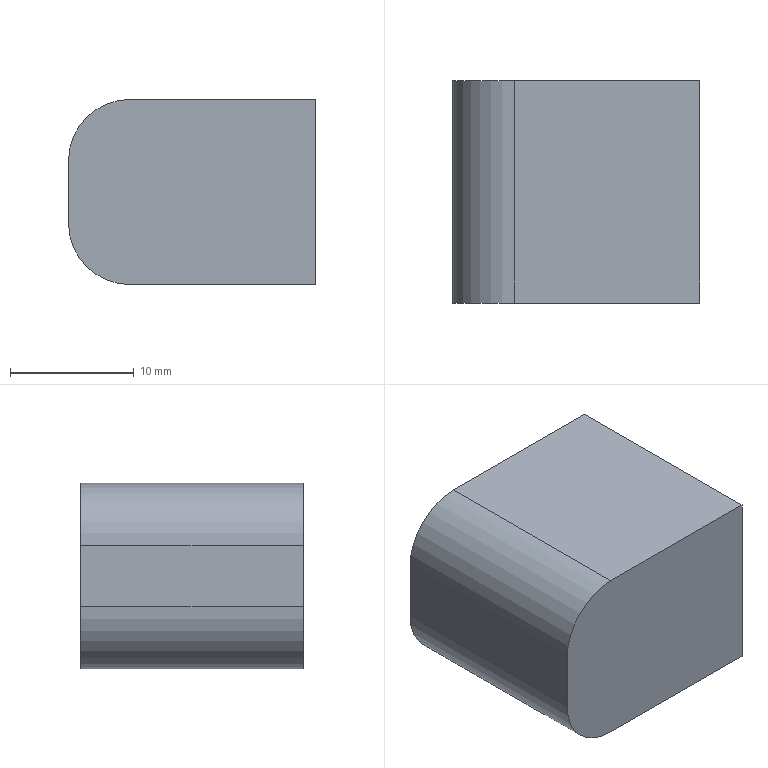Part | STEP file | 1 solid | 8 faces | box 20 x 18 x 15 mm | volume 5207 mm3 | plane 6 | cylinder 2 | commonest cylinder face diameters 10 x2
STEP:
#1=CARTESIAN_POINT('',(0.,0.,0.));
#2=DIRECTION('',(0.,0.,1.));
#3=DIRECTION('',(1.,0.,0.));
#4=AXIS2_PLACEMENT_3D('',#1,#2,#3);
#5=CARTESIAN_POINT('',(-163.106,200.5,167.951));
#6=VERTEX_POINT('',#5);
#7=CARTESIAN_POINT('',(-148.106,200.5,167.951));
#8=VERTEX_POINT('',#7);
#9=CARTESIAN_POINT('',(-72.862,200.5,167.951));
#10=DIRECTION('',(1.,0.,0.));
#11=VECTOR('',#10,1.);
#12=LINE('',#9,#11);
#13=CARTESIAN_POINT('',(-150.606,236.5,167.951));
#14=DIRECTION('',(0.,0.,1.));
#15=DIRECTION('',(1.,0.,0.));
#16=AXIS2_PLACEMENT_3D('',#13,#14,#15);
#17=PLANE('',#16);
#18=CARTESIAN_POINT('',(77.744,-36.));
#19=DIRECTION('',(1.,0.));
#20=VECTOR('',#19,1.);
#21=LINE('',#18,#20);
#22=(GEOMETRIC_REPRESENTATION_CONTEXT(2)PARAMETRIC_REPRESENTATION_CONTEXT()REPRESENTATION_CONTEXT('',''));
#23=DEFINITIONAL_REPRESENTATION('',(#21),#22);
#24=PCURVE('',#17,#23);
#25=CARTESIAN_POINT('',(-72.862,200.5,-363.47));
#26=DIRECTION('',(0.,1.,0.));
#27=DIRECTION('',(0.,0.,-1.));
#28=AXIS2_PLACEMENT_3D('',#25,#26,#27);
#29=PLANE('',#28);
#30=CARTESIAN_POINT('',(-531.422,0.));
#31=DIRECTION('',(0.,-1.));
#32=VECTOR('',#31,1.);
#33=LINE('',#30,#32);
#34=(GEOMETRIC_REPRESENTATION_CONTEXT(2)PARAMETRIC_REPRESENTATION_CONTEXT()REPRESENTATION_CONTEXT('',''));
#35=DEFINITIONAL_REPRESENTATION('',(#33),#34);
#36=PCURVE('',#29,#35);
#37=SURFACE_CURVE('',#12,(#24,#36),.PCURVE_S1.);
#38=EDGE_CURVE('',#6,#8,#37,.T.);
#39=ORIENTED_EDGE('',*,*,#38,.F.);
#40=CARTESIAN_POINT('',(-163.106,182.5,167.951));
#41=VERTEX_POINT('',#40);
#42=CARTESIAN_POINT('',(-163.106,236.5,167.951));
#43=DIRECTION('',(0.,-1.,0.));
#44=VECTOR('',#43,1.);
#45=LINE('',#42,#44);
#46=CARTESIAN_POINT('',(-12.5,0.));
#47=DIRECTION('',(0.,-1.));
#48=VECTOR('',#47,1.);
#49=LINE('',#46,#48);
#50=(GEOMETRIC_REPRESENTATION_CONTEXT(2)PARAMETRIC_REPRESENTATION_CONTEXT()REPRESENTATION_CONTEXT('',''));
#51=DEFINITIONAL_REPRESENTATION('',(#49),#50);
#52=PCURVE('',#17,#51);
#53=CARTESIAN_POINT('',(-163.106,236.5,162.951));
#54=DIRECTION('',(0.,1.,0.));
#55=DIRECTION('',(0.,0.,1.));
#56=AXIS2_PLACEMENT_3D('',#53,#54,#55);
#57=CYLINDRICAL_SURFACE('',#56,5.);
#58=CARTESIAN_POINT('',(6.283,0.));
#59=DIRECTION('',(0.,-1.));
#60=VECTOR('',#59,1.);
#61=LINE('',#58,#60);
#62=(GEOMETRIC_REPRESENTATION_CONTEXT(2)PARAMETRIC_REPRESENTATION_CONTEXT()REPRESENTATION_CONTEXT('',''));
#63=DEFINITIONAL_REPRESENTATION('',(#61),#62);
#64=PCURVE('',#57,#63);
#65=SURFACE_CURVE('',#45,(#52,#64),.PCURVE_S1.);
#66=EDGE_CURVE('',#6,#41,#65,.T.);
#67=ORIENTED_EDGE('',*,*,#66,.T.);
#68=CARTESIAN_POINT('',(-148.106,182.5,167.951));
#69=VERTEX_POINT('',#68);
#70=CARTESIAN_POINT('',(-150.606,182.5,167.951));
#71=DIRECTION('',(-1.,0.,0.));
#72=VECTOR('',#71,1.);
#73=LINE('',#70,#72);
#74=CARTESIAN_POINT('',(0.,-54.));
#75=DIRECTION('',(-1.,0.));
#76=VECTOR('',#75,1.);
#77=LINE('',#74,#76);
#78=(GEOMETRIC_REPRESENTATION_CONTEXT(2)PARAMETRIC_REPRESENTATION_CONTEXT()REPRESENTATION_CONTEXT('',''));
#79=DEFINITIONAL_REPRESENTATION('',(#77),#78);
#80=PCURVE('',#17,#79);
#81=CARTESIAN_POINT('',(-150.606,182.5,152.951));
#82=DIRECTION('',(0.,-1.,0.));
#83=DIRECTION('',(0.,0.,-1.));
#84=AXIS2_PLACEMENT_3D('',#81,#82,#83);
#85=PLANE('',#84);
#86=CARTESIAN_POINT('',(-15.,0.));
#87=DIRECTION('',(0.,-1.));
#88=VECTOR('',#87,1.);
#89=LINE('',#86,#88);
#90=(GEOMETRIC_REPRESENTATION_CONTEXT(2)PARAMETRIC_REPRESENTATION_CONTEXT()REPRESENTATION_CONTEXT('',''));
#91=DEFINITIONAL_REPRESENTATION('',(#89),#90);
#92=PCURVE('',#85,#91);
#93=SURFACE_CURVE('',#73,(#80,#92),.PCURVE_S1.);
#94=EDGE_CURVE('',#69,#41,#93,.T.);
#95=ORIENTED_EDGE('',*,*,#94,.F.);
#96=CARTESIAN_POINT('',(-148.106,236.5,167.951));
#97=DIRECTION('',(0.,-1.,0.));
#98=VECTOR('',#97,1.);
#99=LINE('',#96,#98);
#100=CARTESIAN_POINT('',(2.5,0.));
#101=DIRECTION('',(0.,-1.));
#102=VECTOR('',#101,1.);
#103=LINE('',#100,#102);
#104=(GEOMETRIC_REPRESENTATION_CONTEXT(2)PARAMETRIC_REPRESENTATION_CONTEXT()REPRESENTATION_CONTEXT('',''));
#105=DEFINITIONAL_REPRESENTATION('',(#103),#104);
#106=PCURVE('',#17,#105);
#107=CARTESIAN_POINT('',(-148.106,236.5,152.951));
#108=DIRECTION('',(1.,0.,0.));
#109=DIRECTION('',(0.,0.,-1.));
#110=AXIS2_PLACEMENT_3D('',#107,#108,#109);
#111=PLANE('',#110);
#112=CARTESIAN_POINT('',(-15.,0.));
#113=DIRECTION('',(0.,-1.));
#114=VECTOR('',#113,1.);
#115=LINE('',#112,#114);
#116=(GEOMETRIC_REPRESENTATION_CONTEXT(2)PARAMETRIC_REPRESENTATION_CONTEXT()REPRESENTATION_CONTEXT('',''));
#117=DEFINITIONAL_REPRESENTATION('',(#115),#116);
#118=PCURVE('',#111,#117);
#119=SURFACE_CURVE('',#99,(#106,#118),.PCURVE_S1.);
#120=EDGE_CURVE('',#8,#69,#119,.T.);
#121=ORIENTED_EDGE('',*,*,#120,.F.);
#122=EDGE_LOOP('',(#39,#67,#95,#121));
#123=FACE_BOUND('',#122,.T.);
#124=ADVANCED_FACE('',(#123),#17,.T.);
#125=ORIENTED_EDGE('',*,*,#94,.T.);
#126=CARTESIAN_POINT('',(-168.106,182.5,162.951));
#127=VERTEX_POINT('',#126);
#128=CARTESIAN_POINT('',(-163.106,182.5,162.951));
#129=DIRECTION('',(0.,-1.,0.));
#130=DIRECTION('',(0.,0.,-1.));
#131=AXIS2_PLACEMENT_3D('',#128,#129,#130);
#132=CIRCLE('',#131,5.);
#133=CARTESIAN_POINT('',(-10.,-12.5));
#134=DIRECTION('',(1.,0.));
#135=AXIS2_PLACEMENT_2D('',#133,#134);
#136=CIRCLE('',#135,5.);
#137=(GEOMETRIC_REPRESENTATION_CONTEXT(2)PARAMETRIC_REPRESENTATION_CONTEXT()REPRESENTATION_CONTEXT('',''));
#138=DEFINITIONAL_REPRESENTATION('',(#136),#137);
#139=PCURVE('',#85,#138);
#140=CARTESIAN_POINT('',(9.425,-54.));
#141=DIRECTION('',(-1.,0.));
#142=VECTOR('',#141,1.);
#143=LINE('',#140,#142);
#144=(GEOMETRIC_REPRESENTATION_CONTEXT(2)PARAMETRIC_REPRESENTATION_CONTEXT()REPRESENTATION_CONTEXT('',''));
#145=DEFINITIONAL_REPRESENTATION('',(#143),#144);
#146=PCURVE('',#57,#145);
#147=SURFACE_CURVE('',#132,(#139,#146),.PCURVE_S1.);
#148=EDGE_CURVE('',#41,#127,#147,.T.);
#149=ORIENTED_EDGE('',*,*,#148,.T.);
#150=CARTESIAN_POINT('',(-168.106,182.5,157.951));
#151=VERTEX_POINT('',#150);
#152=CARTESIAN_POINT('',(-168.106,182.5,152.951));
#153=DIRECTION('',(0.,0.,1.));
#154=VECTOR('',#153,1.);
#155=LINE('',#152,#154);
#156=CARTESIAN_POINT('',(0.,-17.5));
#157=DIRECTION('',(-1.,0.));
#158=VECTOR('',#157,1.);
#159=LINE('',#156,#158);
#160=(GEOMETRIC_REPRESENTATION_CONTEXT(2)PARAMETRIC_REPRESENTATION_CONTEXT()REPRESENTATION_CONTEXT('',''));
#161=DEFINITIONAL_REPRESENTATION('',(#159),#160);
#162=PCURVE('',#85,#161);
#163=CARTESIAN_POINT('',(-168.106,236.5,152.951));
#164=DIRECTION('',(-1.,0.,0.));
#165=DIRECTION('',(0.,0.,1.));
#166=AXIS2_PLACEMENT_3D('',#163,#164,#165);
#167=PLANE('',#166);
#168=CARTESIAN_POINT('',(0.,-54.));
#169=DIRECTION('',(1.,0.));
#170=VECTOR('',#169,1.);
#171=LINE('',#168,#170);
#172=(GEOMETRIC_REPRESENTATION_CONTEXT(2)PARAMETRIC_REPRESENTATION_CONTEXT()REPRESENTATION_CONTEXT('',''));
#173=DEFINITIONAL_REPRESENTATION('',(#171),#172);
#174=PCURVE('',#167,#173);
#175=SURFACE_CURVE('',#155,(#162,#174),.PCURVE_S1.);
#176=EDGE_CURVE('',#151,#127,#175,.T.);
#177=ORIENTED_EDGE('',*,*,#176,.F.);
#178=CARTESIAN_POINT('',(-163.106,182.5,152.951));
#179=VERTEX_POINT('',#178);
#180=CARTESIAN_POINT('',(-163.106,182.5,157.951));
#181=DIRECTION('',(0.,-1.,0.));
#182=DIRECTION('',(0.,0.,-1.));
#183=AXIS2_PLACEMENT_3D('',#180,#181,#182);
#184=CIRCLE('',#183,5.);
#185=CARTESIAN_POINT('',(-5.,-12.5));
#186=DIRECTION('',(1.,0.));
#187=AXIS2_PLACEMENT_2D('',#185,#186);
#188=CIRCLE('',#187,5.);
#189=(GEOMETRIC_REPRESENTATION_CONTEXT(2)PARAMETRIC_REPRESENTATION_CONTEXT()REPRESENTATION_CONTEXT('',''));
#190=DEFINITIONAL_REPRESENTATION('',(#188),#189);
#191=PCURVE('',#85,#190);
#192=CARTESIAN_POINT('',(-163.106,236.5,157.951));
#193=DIRECTION('',(0.,-1.,0.));
#194=DIRECTION('',(0.,0.,-1.));
#195=AXIS2_PLACEMENT_3D('',#192,#193,#194);
#196=CYLINDRICAL_SURFACE('',#195,5.);
#197=CARTESIAN_POINT('',(0.,54.));
#198=DIRECTION('',(1.,0.));
#199=VECTOR('',#198,1.);
#200=LINE('',#197,#199);
#201=(GEOMETRIC_REPRESENTATION_CONTEXT(2)PARAMETRIC_REPRESENTATION_CONTEXT()REPRESENTATION_CONTEXT('',''));
#202=DEFINITIONAL_REPRESENTATION('',(#200),#201);
#203=PCURVE('',#196,#202);
#204=SURFACE_CURVE('',#184,(#191,#203),.PCURVE_S1.);
#205=EDGE_CURVE('',#151,#179,#204,.T.);
#206=ORIENTED_EDGE('',*,*,#205,.T.);
#207=CARTESIAN_POINT('',(-148.106,182.5,152.951));
#208=VERTEX_POINT('',#207);
#209=CARTESIAN_POINT('',(-150.606,182.5,152.951));
#210=DIRECTION('',(1.,0.,0.));
#211=VECTOR('',#210,1.);
#212=LINE('',#209,#211);
#213=CARTESIAN_POINT('',(0.,0.));
#214=DIRECTION('',(0.,1.));
#215=VECTOR('',#214,1.);
#216=LINE('',#213,#215);
#217=(GEOMETRIC_REPRESENTATION_CONTEXT(2)PARAMETRIC_REPRESENTATION_CONTEXT()REPRESENTATION_CONTEXT('',''));
#218=DEFINITIONAL_REPRESENTATION('',(#216),#217);
#219=PCURVE('',#85,#218);
#220=CARTESIAN_POINT('',(-150.606,236.5,152.951));
#221=DIRECTION('',(0.,0.,-1.));
#222=DIRECTION('',(-1.,0.,0.));
#223=AXIS2_PLACEMENT_3D('',#220,#221,#222);
#224=PLANE('',#223);
#225=CARTESIAN_POINT('',(0.,-54.));
#226=DIRECTION('',(-1.,0.));
#227=VECTOR('',#226,1.);
#228=LINE('',#225,#227);
#229=(GEOMETRIC_REPRESENTATION_CONTEXT(2)PARAMETRIC_REPRESENTATION_CONTEXT()REPRESENTATION_CONTEXT('',''));
#230=DEFINITIONAL_REPRESENTATION('',(#228),#229);
#231=PCURVE('',#224,#230);
#232=SURFACE_CURVE('',#212,(#219,#231),.PCURVE_S1.);
#233=EDGE_CURVE('',#179,#208,#232,.T.);
#234=ORIENTED_EDGE('',*,*,#233,.T.);
#235=CARTESIAN_POINT('',(-148.106,182.5,152.951));
#236=DIRECTION('',(0.,0.,1.));
#237=VECTOR('',#236,1.);
#238=LINE('',#235,#237);
#239=CARTESIAN_POINT('',(0.,2.5));
#240=DIRECTION('',(-1.,0.));
#241=VECTOR('',#240,1.);
#242=LINE('',#239,#241);
#243=(GEOMETRIC_REPRESENTATION_CONTEXT(2)PARAMETRIC_REPRESENTATION_CONTEXT()REPRESENTATION_CONTEXT('',''));
#244=DEFINITIONAL_REPRESENTATION('',(#242),#243);
#245=PCURVE('',#85,#244);
#246=CARTESIAN_POINT('',(0.,-54.));
#247=DIRECTION('',(-1.,0.));
#248=VECTOR('',#247,1.);
#249=LINE('',#246,#248);
#250=(GEOMETRIC_REPRESENTATION_CONTEXT(2)PARAMETRIC_REPRESENTATION_CONTEXT()REPRESENTATION_CONTEXT('',''));
#251=DEFINITIONAL_REPRESENTATION('',(#249),#250);
#252=PCURVE('',#111,#251);
#253=SURFACE_CURVE('',#238,(#245,#252),.PCURVE_S1.);
#254=EDGE_CURVE('',#208,#69,#253,.T.);
#255=ORIENTED_EDGE('',*,*,#254,.T.);
#256=EDGE_LOOP('',(#125,#149,#177,#206,#234,#255));
#257=FACE_BOUND('',#256,.T.);
#258=ADVANCED_FACE('',(#257),#85,.T.);
#259=ORIENTED_EDGE('',*,*,#176,.T.);
#260=CARTESIAN_POINT('',(-168.106,200.5,162.951));
#261=VERTEX_POINT('',#260);
#262=CARTESIAN_POINT('',(-168.106,236.5,162.951));
#263=DIRECTION('',(0.,1.,0.));
#264=VECTOR('',#263,1.);
#265=LINE('',#262,#264);
#266=CARTESIAN_POINT('',(10.,0.));
#267=DIRECTION('',(0.,1.));
#268=VECTOR('',#267,1.);
#269=LINE('',#266,#268);
#270=(GEOMETRIC_REPRESENTATION_CONTEXT(2)PARAMETRIC_REPRESENTATION_CONTEXT()REPRESENTATION_CONTEXT('',''));
#271=DEFINITIONAL_REPRESENTATION('',(#269),#270);
#272=PCURVE('',#167,#271);
#273=CARTESIAN_POINT('',(4.712,0.));
#274=DIRECTION('',(0.,1.));
#275=VECTOR('',#274,1.);
#276=LINE('',#273,#275);
#277=(GEOMETRIC_REPRESENTATION_CONTEXT(2)PARAMETRIC_REPRESENTATION_CONTEXT()REPRESENTATION_CONTEXT('',''));
#278=DEFINITIONAL_REPRESENTATION('',(#276),#277);
#279=PCURVE('',#57,#278);
#280=SURFACE_CURVE('',#265,(#272,#279),.PCURVE_S1.);
#281=EDGE_CURVE('',#127,#261,#280,.T.);
#282=ORIENTED_EDGE('',*,*,#281,.T.);
#283=CARTESIAN_POINT('',(-168.106,200.5,157.951));
#284=VERTEX_POINT('',#283);
#285=CARTESIAN_POINT('',(-168.106,200.5,-363.47));
#286=DIRECTION('',(0.,0.,1.));
#287=VECTOR('',#286,1.);
#288=LINE('',#285,#287);
#289=CARTESIAN_POINT('',(-516.422,-36.));
#290=DIRECTION('',(1.,0.));
#291=VECTOR('',#290,1.);
#292=LINE('',#289,#291);
#293=(GEOMETRIC_REPRESENTATION_CONTEXT(2)PARAMETRIC_REPRESENTATION_CONTEXT()REPRESENTATION_CONTEXT('',''));
#294=DEFINITIONAL_REPRESENTATION('',(#292),#293);
#295=PCURVE('',#167,#294);
#296=CARTESIAN_POINT('',(0.,95.244));
#297=DIRECTION('',(-1.,0.));
#298=VECTOR('',#297,1.);
#299=LINE('',#296,#298);
#300=(GEOMETRIC_REPRESENTATION_CONTEXT(2)PARAMETRIC_REPRESENTATION_CONTEXT()REPRESENTATION_CONTEXT('',''));
#301=DEFINITIONAL_REPRESENTATION('',(#299),#300);
#302=PCURVE('',#29,#301);
#303=SURFACE_CURVE('',#288,(#295,#302),.PCURVE_S1.);
#304=EDGE_CURVE('',#284,#261,#303,.T.);
#305=ORIENTED_EDGE('',*,*,#304,.F.);
#306=CARTESIAN_POINT('',(-168.106,236.5,157.951));
#307=DIRECTION('',(0.,-1.,0.));
#308=VECTOR('',#307,1.);
#309=LINE('',#306,#308);
#310=CARTESIAN_POINT('',(5.,0.));
#311=DIRECTION('',(0.,-1.));
#312=VECTOR('',#311,1.);
#313=LINE('',#310,#312);
#314=(GEOMETRIC_REPRESENTATION_CONTEXT(2)PARAMETRIC_REPRESENTATION_CONTEXT()REPRESENTATION_CONTEXT('',''));
#315=DEFINITIONAL_REPRESENTATION('',(#313),#314);
#316=PCURVE('',#167,#315);
#317=CARTESIAN_POINT('',(4.712,0.));
#318=DIRECTION('',(0.,1.));
#319=VECTOR('',#318,1.);
#320=LINE('',#317,#319);
#321=(GEOMETRIC_REPRESENTATION_CONTEXT(2)PARAMETRIC_REPRESENTATION_CONTEXT()REPRESENTATION_CONTEXT('',''));
#322=DEFINITIONAL_REPRESENTATION('',(#320),#321);
#323=PCURVE('',#196,#322);
#324=SURFACE_CURVE('',#309,(#316,#323),.PCURVE_S1.);
#325=EDGE_CURVE('',#284,#151,#324,.T.);
#326=ORIENTED_EDGE('',*,*,#325,.T.);
#327=EDGE_LOOP('',(#259,#282,#305,#326));
#328=FACE_BOUND('',#327,.T.);
#329=ADVANCED_FACE('',(#328),#167,.T.);
#330=ORIENTED_EDGE('',*,*,#304,.T.);
#331=CARTESIAN_POINT('',(-163.106,200.5,162.951));
#332=DIRECTION('',(0.,1.,0.));
#333=DIRECTION('',(0.,0.,1.));
#334=AXIS2_PLACEMENT_3D('',#331,#332,#333);
#335=CIRCLE('',#334,5.);
#336=CARTESIAN_POINT('',(-526.422,90.244));
#337=DIRECTION('',(-1.,0.));
#338=AXIS2_PLACEMENT_2D('',#336,#337);
#339=CIRCLE('',#338,5.);
#340=(GEOMETRIC_REPRESENTATION_CONTEXT(2)PARAMETRIC_REPRESENTATION_CONTEXT()REPRESENTATION_CONTEXT('',''));
#341=DEFINITIONAL_REPRESENTATION('',(#339),#340);
#342=PCURVE('',#29,#341);
#343=CARTESIAN_POINT('',(0.,-36.));
#344=DIRECTION('',(1.,0.));
#345=VECTOR('',#344,1.);
#346=LINE('',#343,#345);
#347=(GEOMETRIC_REPRESENTATION_CONTEXT(2)PARAMETRIC_REPRESENTATION_CONTEXT()REPRESENTATION_CONTEXT('',''));
#348=DEFINITIONAL_REPRESENTATION('',(#346),#347);
#349=PCURVE('',#57,#348);
#350=SURFACE_CURVE('',#335,(#342,#349),.PCURVE_S1.);
#351=EDGE_CURVE('',#261,#6,#350,.T.);
#352=ORIENTED_EDGE('',*,*,#351,.T.);
#353=ORIENTED_EDGE('',*,*,#38,.T.);
#354=CARTESIAN_POINT('',(-148.106,200.5,152.951));
#355=VERTEX_POINT('',#354);
#356=CARTESIAN_POINT('',(-148.106,200.5,152.951));
#357=DIRECTION('',(0.,0.,1.));
#358=VECTOR('',#357,1.);
#359=LINE('',#356,#358);
#360=CARTESIAN_POINT('',(-516.422,75.244));
#361=DIRECTION('',(-1.,0.));
#362=VECTOR('',#361,1.);
#363=LINE('',#360,#362);
#364=(GEOMETRIC_REPRESENTATION_CONTEXT(2)PARAMETRIC_REPRESENTATION_CONTEXT()REPRESENTATION_CONTEXT('',''));
#365=DEFINITIONAL_REPRESENTATION('',(#363),#364);
#366=PCURVE('',#29,#365);
#367=CARTESIAN_POINT('',(0.,-36.));
#368=DIRECTION('',(-1.,0.));
#369=VECTOR('',#368,1.);
#370=LINE('',#367,#369);
#371=(GEOMETRIC_REPRESENTATION_CONTEXT(2)PARAMETRIC_REPRESENTATION_CONTEXT()REPRESENTATION_CONTEXT('',''));
#372=DEFINITIONAL_REPRESENTATION('',(#370),#371);
#373=PCURVE('',#111,#372);
#374=SURFACE_CURVE('',#359,(#366,#373),.PCURVE_S1.);
#375=EDGE_CURVE('',#355,#8,#374,.T.);
#376=ORIENTED_EDGE('',*,*,#375,.F.);
#377=CARTESIAN_POINT('',(-163.106,200.5,152.951));
#378=VERTEX_POINT('',#377);
#379=CARTESIAN_POINT('',(-72.862,200.5,152.951));
#380=DIRECTION('',(-1.,0.,0.));
#381=VECTOR('',#380,1.);
#382=LINE('',#379,#381);
#383=CARTESIAN_POINT('',(-516.422,0.));
#384=DIRECTION('',(0.,1.));
#385=VECTOR('',#384,1.);
#386=LINE('',#383,#385);
#387=(GEOMETRIC_REPRESENTATION_CONTEXT(2)PARAMETRIC_REPRESENTATION_CONTEXT()REPRESENTATION_CONTEXT('',''));
#388=DEFINITIONAL_REPRESENTATION('',(#386),#387);
#389=PCURVE('',#29,#388);
#390=CARTESIAN_POINT('',(-77.744,-36.));
#391=DIRECTION('',(1.,0.));
#392=VECTOR('',#391,1.);
#393=LINE('',#390,#392);
#394=(GEOMETRIC_REPRESENTATION_CONTEXT(2)PARAMETRIC_REPRESENTATION_CONTEXT()REPRESENTATION_CONTEXT('',''));
#395=DEFINITIONAL_REPRESENTATION('',(#393),#394);
#396=PCURVE('',#224,#395);
#397=SURFACE_CURVE('',#382,(#389,#396),.PCURVE_S1.);
#398=EDGE_CURVE('',#355,#378,#397,.T.);
#399=ORIENTED_EDGE('',*,*,#398,.T.);
#400=CARTESIAN_POINT('',(-163.106,200.5,157.951));
#401=DIRECTION('',(0.,1.,0.));
#402=DIRECTION('',(0.,0.,1.));
#403=AXIS2_PLACEMENT_3D('',#400,#401,#402);
#404=CIRCLE('',#403,5.);
#405=CARTESIAN_POINT('',(-521.422,90.244));
#406=DIRECTION('',(-1.,0.));
#407=AXIS2_PLACEMENT_2D('',#405,#406);
#408=CIRCLE('',#407,5.);
#409=(GEOMETRIC_REPRESENTATION_CONTEXT(2)PARAMETRIC_REPRESENTATION_CONTEXT()REPRESENTATION_CONTEXT('',''));
#410=DEFINITIONAL_REPRESENTATION('',(#408),#409);
#411=PCURVE('',#29,#410);
#412=CARTESIAN_POINT('',(9.425,36.));
#413=DIRECTION('',(-1.,0.));
#414=VECTOR('',#413,1.);
#415=LINE('',#412,#414);
#416=(GEOMETRIC_REPRESENTATION_CONTEXT(2)PARAMETRIC_REPRESENTATION_CONTEXT()REPRESENTATION_CONTEXT('',''));
#417=DEFINITIONAL_REPRESENTATION('',(#415),#416);
#418=PCURVE('',#196,#417);
#419=SURFACE_CURVE('',#404,(#411,#418),.PCURVE_S1.);
#420=EDGE_CURVE('',#378,#284,#419,.T.);
#421=ORIENTED_EDGE('',*,*,#420,.T.);
#422=EDGE_LOOP('',(#330,#352,#353,#376,#399,#421));
#423=FACE_BOUND('',#422,.T.);
#424=ADVANCED_FACE('',(#423),#29,.T.);
#425=ORIENTED_EDGE('',*,*,#233,.F.);
#426=CARTESIAN_POINT('',(-163.106,236.5,152.951));
#427=DIRECTION('',(0.,1.,0.));
#428=VECTOR('',#427,1.);
#429=LINE('',#426,#428);
#430=CARTESIAN_POINT('',(12.5,0.));
#431=DIRECTION('',(0.,1.));
#432=VECTOR('',#431,1.);
#433=LINE('',#430,#432);
#434=(GEOMETRIC_REPRESENTATION_CONTEXT(2)PARAMETRIC_REPRESENTATION_CONTEXT()REPRESENTATION_CONTEXT('',''));
#435=DEFINITIONAL_REPRESENTATION('',(#433),#434);
#436=PCURVE('',#224,#435);
#437=CARTESIAN_POINT('',(6.283,0.));
#438=DIRECTION('',(0.,-1.));
#439=VECTOR('',#438,1.);
#440=LINE('',#437,#439);
#441=(GEOMETRIC_REPRESENTATION_CONTEXT(2)PARAMETRIC_REPRESENTATION_CONTEXT()REPRESENTATION_CONTEXT('',''));
#442=DEFINITIONAL_REPRESENTATION('',(#440),#441);
#443=PCURVE('',#196,#442);
#444=SURFACE_CURVE('',#429,(#436,#443),.PCURVE_S1.);
#445=EDGE_CURVE('',#179,#378,#444,.T.);
#446=ORIENTED_EDGE('',*,*,#445,.T.);
#447=ORIENTED_EDGE('',*,*,#398,.F.);
#448=CARTESIAN_POINT('',(-148.106,236.5,152.951));
#449=DIRECTION('',(0.,1.,0.));
#450=VECTOR('',#449,1.);
#451=LINE('',#448,#450);
#452=CARTESIAN_POINT('',(-2.5,0.));
#453=DIRECTION('',(0.,1.));
#454=VECTOR('',#453,1.);
#455=LINE('',#452,#454);
#456=(GEOMETRIC_REPRESENTATION_CONTEXT(2)PARAMETRIC_REPRESENTATION_CONTEXT()REPRESENTATION_CONTEXT('',''));
#457=DEFINITIONAL_REPRESENTATION('',(#455),#456);
#458=PCURVE('',#224,#457);
#459=CARTESIAN_POINT('',(0.,0.));
#460=DIRECTION('',(0.,1.));
#461=VECTOR('',#460,1.);
#462=LINE('',#459,#461);
#463=(GEOMETRIC_REPRESENTATION_CONTEXT(2)PARAMETRIC_REPRESENTATION_CONTEXT()REPRESENTATION_CONTEXT('',''));
#464=DEFINITIONAL_REPRESENTATION('',(#462),#463);
#465=PCURVE('',#111,#464);
#466=SURFACE_CURVE('',#451,(#458,#465),.PCURVE_S1.);
#467=EDGE_CURVE('',#208,#355,#466,.T.);
#468=ORIENTED_EDGE('',*,*,#467,.F.);
#469=EDGE_LOOP('',(#425,#446,#447,#468));
#470=FACE_BOUND('',#469,.T.);
#471=ADVANCED_FACE('',(#470),#224,.T.);
#472=ORIENTED_EDGE('',*,*,#467,.T.);
#473=ORIENTED_EDGE('',*,*,#375,.T.);
#474=ORIENTED_EDGE('',*,*,#120,.T.);
#475=ORIENTED_EDGE('',*,*,#254,.F.);
#476=EDGE_LOOP('',(#472,#473,#474,#475));
#477=FACE_BOUND('',#476,.T.);
#478=ADVANCED_FACE('',(#477),#111,.T.);
#479=ORIENTED_EDGE('',*,*,#148,.F.);
#480=ORIENTED_EDGE('',*,*,#66,.F.);
#481=ORIENTED_EDGE('',*,*,#351,.F.);
#482=ORIENTED_EDGE('',*,*,#281,.F.);
#483=EDGE_LOOP('',(#479,#480,#481,#482));
#484=FACE_BOUND('',#483,.T.);
#485=ADVANCED_FACE('',(#484),#57,.T.);
#486=ORIENTED_EDGE('',*,*,#420,.F.);
#487=ORIENTED_EDGE('',*,*,#445,.F.);
#488=ORIENTED_EDGE('',*,*,#205,.F.);
#489=ORIENTED_EDGE('',*,*,#325,.F.);
#490=EDGE_LOOP('',(#486,#487,#488,#489));
#491=FACE_BOUND('',#490,.T.);
#492=ADVANCED_FACE('',(#491),#196,.T.);
#493=CLOSED_SHELL('',(#124,#258,#329,#424,#471,#478,#485,#492));
#494=MANIFOLD_SOLID_BREP('',#493);
#495=(LENGTH_UNIT()NAMED_UNIT(*)SI_UNIT(.MILLI.,.METRE.));
#496=UNCERTAINTY_MEASURE_WITH_UNIT(LENGTH_MEASURE(0.0000001),#495,'','');
#497=(NAMED_UNIT(*)PLANE_ANGLE_UNIT()SI_UNIT($,.RADIAN.));
#498=(NAMED_UNIT(*)SI_UNIT($,.STERADIAN.)SOLID_ANGLE_UNIT());
#499=(GEOMETRIC_REPRESENTATION_CONTEXT(3)GLOBAL_UNCERTAINTY_ASSIGNED_CONTEXT((#496))GLOBAL_UNIT_ASSIGNED_CONTEXT((#495,#497,#498))REPRESENTATION_CONTEXT('',''));
#500=ADVANCED_BREP_SHAPE_REPRESENTATION('',(#4,#494),#499);